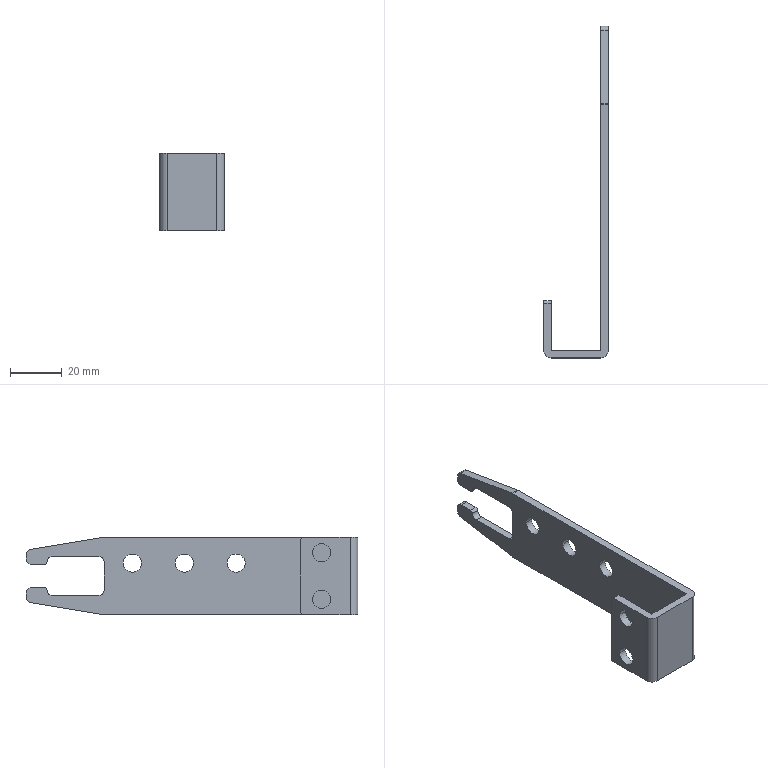Part | STEP file | 13 | 1 solid | 46 faces | box 25 x 128 x 30 mm | volume 12857 mm3 | cylinder 28 | plane 18 | commonest cylinder face diameters 4 x10 7 x10 2 x4 0.02 x2 6.02 x2